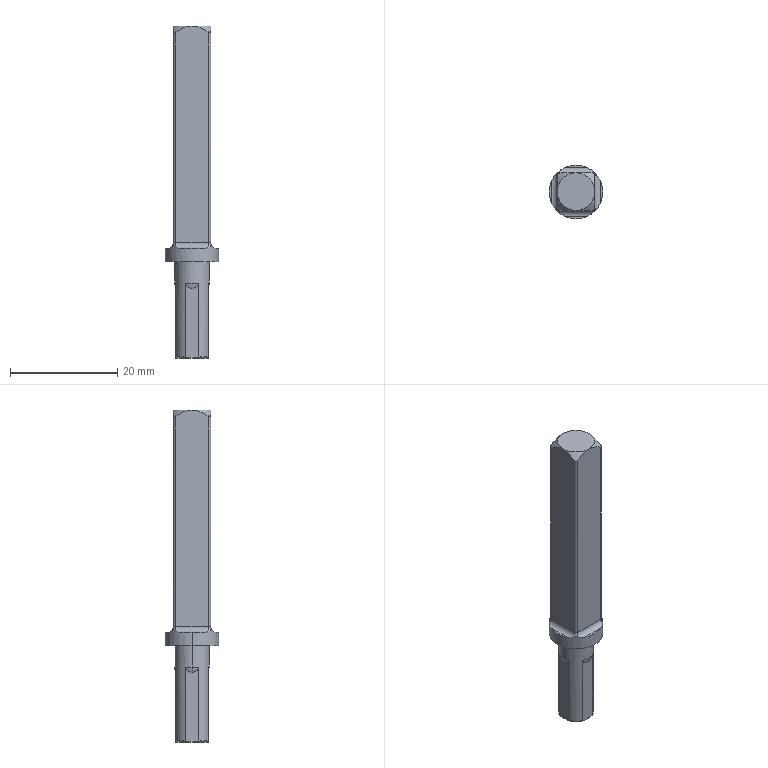Part | SolidWorks | features Fillet 3, ICE 3, Extrusion 1, HoleWzd 1, RevCut 1 | 1 solid | 49 faces | box 10 x 10 x 62 mm | volume 2691 mm3 | plane 15 | cylinder 14 | cone 10 | torus 6 | spline 4 | commonest cylinder face diameters 1 x4 2 x4 3.3 x2 6.5 x2 10 x2